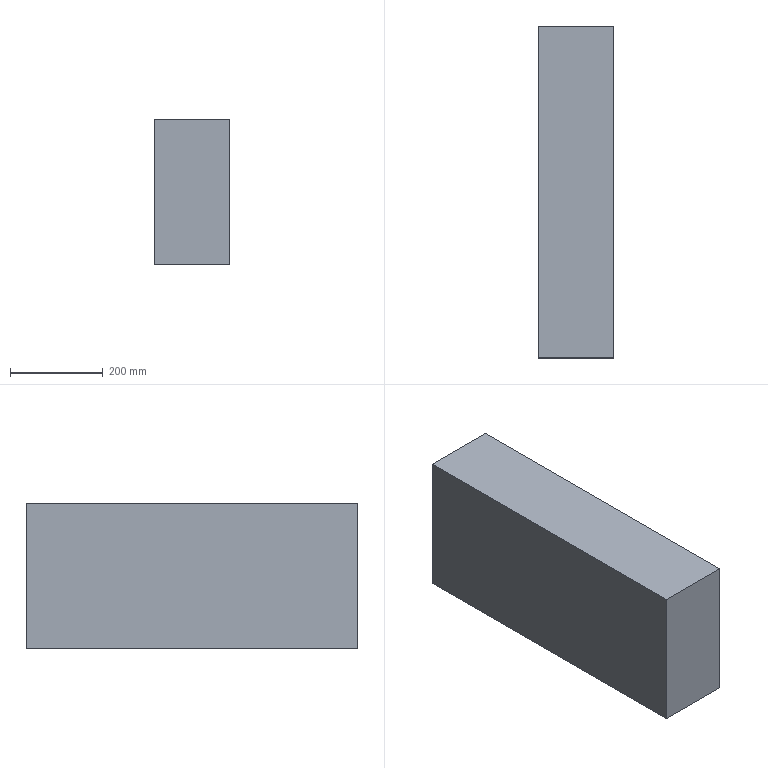Part | STEP file | 1 solid | 6 faces | box 162.496 x 714.237 x 313.918 mm | volume 36433685 mm3 | plane 6
STEP:
#1=CARTESIAN_POINT('',(0.,0.,0.));
#2=DIRECTION('',(0.,0.,1.));
#3=DIRECTION('',(1.,0.,0.));
#4=AXIS2_PLACEMENT_3D('',#1,#2,#3);
#5=CARTESIAN_POINT('',(-762.496,164.237,-106.359));
#6=VERTEX_POINT('',#5);
#7=CARTESIAN_POINT('',(-762.496,164.237,207.559));
#8=VERTEX_POINT('',#7);
#9=CARTESIAN_POINT('',(-762.496,164.237,-106.359));
#10=DIRECTION('',(0.,0.,1.));
#11=VECTOR('',#10,1.);
#12=LINE('',#9,#11);
#13=CARTESIAN_POINT('',(-762.496,164.237,207.569));
#14=DIRECTION('',(1.,0.,0.));
#15=DIRECTION('',(0.,0.,-1.));
#16=AXIS2_PLACEMENT_3D('',#13,#14,#15);
#17=PLANE('',#16);
#18=CARTESIAN_POINT('',(313.928,0.));
#19=DIRECTION('',(-1.,0.));
#20=VECTOR('',#19,1.);
#21=LINE('',#18,#20);
#22=(GEOMETRIC_REPRESENTATION_CONTEXT(2)PARAMETRIC_REPRESENTATION_CONTEXT()REPRESENTATION_CONTEXT('',''));
#23=DEFINITIONAL_REPRESENTATION('',(#21),#22);
#24=PCURVE('',#17,#23);
#25=CARTESIAN_POINT('',(-812.,164.237,-106.359));
#26=DIRECTION('',(0.,-1.,0.));
#27=DIRECTION('',(0.,0.,-1.));
#28=AXIS2_PLACEMENT_3D('',#25,#26,#27);
#29=PLANE('',#28);
#30=CARTESIAN_POINT('',(0.,49.504));
#31=DIRECTION('',(-1.,0.));
#32=VECTOR('',#31,1.);
#33=LINE('',#30,#32);
#34=(GEOMETRIC_REPRESENTATION_CONTEXT(2)PARAMETRIC_REPRESENTATION_CONTEXT()REPRESENTATION_CONTEXT('',''));
#35=DEFINITIONAL_REPRESENTATION('',(#33),#34);
#36=PCURVE('',#29,#35);
#37=SURFACE_CURVE('',#12,(#24,#36),.PCURVE_S1.);
#38=EDGE_CURVE('',#6,#8,#37,.T.);
#39=ORIENTED_EDGE('',*,*,#38,.F.);
#40=CARTESIAN_POINT('',(-762.496,-550.,-106.359));
#41=VERTEX_POINT('',#40);
#42=CARTESIAN_POINT('',(-762.496,-550.,-106.359));
#43=DIRECTION('',(0.,1.,0.));
#44=VECTOR('',#43,1.);
#45=LINE('',#42,#44);
#46=CARTESIAN_POINT('',(313.928,-714.237));
#47=DIRECTION('',(0.,1.));
#48=VECTOR('',#47,1.);
#49=LINE('',#46,#48);
#50=(GEOMETRIC_REPRESENTATION_CONTEXT(2)PARAMETRIC_REPRESENTATION_CONTEXT()REPRESENTATION_CONTEXT('',''));
#51=DEFINITIONAL_REPRESENTATION('',(#49),#50);
#52=PCURVE('',#17,#51);
#53=CARTESIAN_POINT('',(-812.,-550.,-106.359));
#54=DIRECTION('',(0.,0.,1.));
#55=DIRECTION('',(1.,0.,0.));
#56=AXIS2_PLACEMENT_3D('',#53,#54,#55);
#57=PLANE('',#56);
#58=CARTESIAN_POINT('',(49.504,0.));
#59=DIRECTION('',(0.,1.));
#60=VECTOR('',#59,1.);
#61=LINE('',#58,#60);
#62=(GEOMETRIC_REPRESENTATION_CONTEXT(2)PARAMETRIC_REPRESENTATION_CONTEXT()REPRESENTATION_CONTEXT('',''));
#63=DEFINITIONAL_REPRESENTATION('',(#61),#62);
#64=PCURVE('',#57,#63);
#65=SURFACE_CURVE('',#45,(#52,#64),.PCURVE_S1.);
#66=EDGE_CURVE('',#41,#6,#65,.T.);
#67=ORIENTED_EDGE('',*,*,#66,.F.);
#68=CARTESIAN_POINT('',(-762.496,-550.,207.559));
#69=VERTEX_POINT('',#68);
#70=CARTESIAN_POINT('',(-762.496,-550.,-106.359));
#71=DIRECTION('',(0.,0.,-1.));
#72=VECTOR('',#71,1.);
#73=LINE('',#70,#72);
#74=CARTESIAN_POINT('',(313.928,-714.237));
#75=DIRECTION('',(1.,0.));
#76=VECTOR('',#75,1.);
#77=LINE('',#74,#76);
#78=(GEOMETRIC_REPRESENTATION_CONTEXT(2)PARAMETRIC_REPRESENTATION_CONTEXT()REPRESENTATION_CONTEXT('',''));
#79=DEFINITIONAL_REPRESENTATION('',(#77),#78);
#80=PCURVE('',#17,#79);
#81=CARTESIAN_POINT('',(-812.,-550.,-106.359));
#82=DIRECTION('',(0.,1.,0.));
#83=DIRECTION('',(0.,0.,1.));
#84=AXIS2_PLACEMENT_3D('',#81,#82,#83);
#85=PLANE('',#84);
#86=CARTESIAN_POINT('',(0.,49.504));
#87=DIRECTION('',(-1.,0.));
#88=VECTOR('',#87,1.);
#89=LINE('',#86,#88);
#90=(GEOMETRIC_REPRESENTATION_CONTEXT(2)PARAMETRIC_REPRESENTATION_CONTEXT()REPRESENTATION_CONTEXT('',''));
#91=DEFINITIONAL_REPRESENTATION('',(#89),#90);
#92=PCURVE('',#85,#91);
#93=SURFACE_CURVE('',#73,(#80,#92),.PCURVE_S1.);
#94=EDGE_CURVE('',#69,#41,#93,.T.);
#95=ORIENTED_EDGE('',*,*,#94,.F.);
#96=CARTESIAN_POINT('',(-762.496,-550.,207.559));
#97=DIRECTION('',(0.,-1.,0.));
#98=VECTOR('',#97,1.);
#99=LINE('',#96,#98);
#100=CARTESIAN_POINT('',(0.01,-714.237));
#101=DIRECTION('',(0.,-1.));
#102=VECTOR('',#101,1.);
#103=LINE('',#100,#102);
#104=(GEOMETRIC_REPRESENTATION_CONTEXT(2)PARAMETRIC_REPRESENTATION_CONTEXT()REPRESENTATION_CONTEXT('',''));
#105=DEFINITIONAL_REPRESENTATION('',(#103),#104);
#106=PCURVE('',#17,#105);
#107=CARTESIAN_POINT('',(-812.,-550.,207.559));
#108=DIRECTION('',(0.,0.,-1.));
#109=DIRECTION('',(-1.,0.,0.));
#110=AXIS2_PLACEMENT_3D('',#107,#108,#109);
#111=PLANE('',#110);
#112=CARTESIAN_POINT('',(-49.504,0.));
#113=DIRECTION('',(0.,-1.));
#114=VECTOR('',#113,1.);
#115=LINE('',#112,#114);
#116=(GEOMETRIC_REPRESENTATION_CONTEXT(2)PARAMETRIC_REPRESENTATION_CONTEXT()REPRESENTATION_CONTEXT('',''));
#117=DEFINITIONAL_REPRESENTATION('',(#115),#116);
#118=PCURVE('',#111,#117);
#119=SURFACE_CURVE('',#99,(#106,#118),.PCURVE_S1.);
#120=EDGE_CURVE('',#8,#69,#119,.T.);
#121=ORIENTED_EDGE('',*,*,#120,.F.);
#122=EDGE_LOOP('',(#39,#67,#95,#121));
#123=FACE_BOUND('',#122,.T.);
#124=ADVANCED_FACE('',(#123),#17,.F.);
#125=CARTESIAN_POINT('',(-600.,164.237,-106.359));
#126=VERTEX_POINT('',#125);
#127=CARTESIAN_POINT('',(-812.,164.237,-106.359));
#128=DIRECTION('',(1.,0.,0.));
#129=VECTOR('',#128,1.);
#130=LINE('',#127,#129);
#131=CARTESIAN_POINT('',(0.,0.));
#132=DIRECTION('',(0.,1.));
#133=VECTOR('',#132,1.);
#134=LINE('',#131,#133);
#135=(GEOMETRIC_REPRESENTATION_CONTEXT(2)PARAMETRIC_REPRESENTATION_CONTEXT()REPRESENTATION_CONTEXT('',''));
#136=DEFINITIONAL_REPRESENTATION('',(#134),#135);
#137=PCURVE('',#29,#136);
#138=CARTESIAN_POINT('',(0.,714.237));
#139=DIRECTION('',(1.,0.));
#140=VECTOR('',#139,1.);
#141=LINE('',#138,#140);
#142=(GEOMETRIC_REPRESENTATION_CONTEXT(2)PARAMETRIC_REPRESENTATION_CONTEXT()REPRESENTATION_CONTEXT('',''));
#143=DEFINITIONAL_REPRESENTATION('',(#141),#142);
#144=PCURVE('',#57,#143);
#145=SURFACE_CURVE('',#130,(#137,#144),.PCURVE_S1.);
#146=EDGE_CURVE('',#6,#126,#145,.T.);
#147=ORIENTED_EDGE('',*,*,#146,.F.);
#148=ORIENTED_EDGE('',*,*,#38,.T.);
#149=CARTESIAN_POINT('',(-600.,164.237,207.559));
#150=VERTEX_POINT('',#149);
#151=CARTESIAN_POINT('',(-812.,164.237,207.559));
#152=DIRECTION('',(1.,0.,0.));
#153=VECTOR('',#152,1.);
#154=LINE('',#151,#153);
#155=CARTESIAN_POINT('',(-313.918,0.));
#156=DIRECTION('',(0.,1.));
#157=VECTOR('',#156,1.);
#158=LINE('',#155,#157);
#159=(GEOMETRIC_REPRESENTATION_CONTEXT(2)PARAMETRIC_REPRESENTATION_CONTEXT()REPRESENTATION_CONTEXT('',''));
#160=DEFINITIONAL_REPRESENTATION('',(#158),#159);
#161=PCURVE('',#29,#160);
#162=CARTESIAN_POINT('',(0.,714.237));
#163=DIRECTION('',(-1.,0.));
#164=VECTOR('',#163,1.);
#165=LINE('',#162,#164);
#166=(GEOMETRIC_REPRESENTATION_CONTEXT(2)PARAMETRIC_REPRESENTATION_CONTEXT()REPRESENTATION_CONTEXT('',''));
#167=DEFINITIONAL_REPRESENTATION('',(#165),#166);
#168=PCURVE('',#111,#167);
#169=SURFACE_CURVE('',#154,(#161,#168),.PCURVE_S1.);
#170=EDGE_CURVE('',#8,#150,#169,.T.);
#171=ORIENTED_EDGE('',*,*,#170,.T.);
#172=CARTESIAN_POINT('',(-600.,164.237,-106.359));
#173=DIRECTION('',(0.,0.,-1.));
#174=VECTOR('',#173,1.);
#175=LINE('',#172,#174);
#176=CARTESIAN_POINT('',(0.,212.));
#177=DIRECTION('',(1.,0.));
#178=VECTOR('',#177,1.);
#179=LINE('',#176,#178);
#180=(GEOMETRIC_REPRESENTATION_CONTEXT(2)PARAMETRIC_REPRESENTATION_CONTEXT()REPRESENTATION_CONTEXT('',''));
#181=DEFINITIONAL_REPRESENTATION('',(#179),#180);
#182=PCURVE('',#29,#181);
#183=CARTESIAN_POINT('',(-600.,0.,0.));
#184=DIRECTION('',(1.,0.,0.));
#185=DIRECTION('',(0.,0.,-1.));
#186=AXIS2_PLACEMENT_3D('',#183,#184,#185);
#187=PLANE('',#186);
#188=CARTESIAN_POINT('',(106.359,164.237));
#189=DIRECTION('',(1.,0.));
#190=VECTOR('',#189,1.);
#191=LINE('',#188,#190);
#192=(GEOMETRIC_REPRESENTATION_CONTEXT(2)PARAMETRIC_REPRESENTATION_CONTEXT()REPRESENTATION_CONTEXT('',''));
#193=DEFINITIONAL_REPRESENTATION('',(#191),#192);
#194=PCURVE('',#187,#193);
#195=SURFACE_CURVE('',#175,(#182,#194),.PCURVE_S1.);
#196=EDGE_CURVE('',#150,#126,#195,.T.);
#197=ORIENTED_EDGE('',*,*,#196,.T.);
#198=EDGE_LOOP('',(#147,#148,#171,#197));
#199=FACE_BOUND('',#198,.T.);
#200=ADVANCED_FACE('',(#199),#29,.F.);
#201=CARTESIAN_POINT('',(-600.,-550.,-106.359));
#202=VERTEX_POINT('',#201);
#203=CARTESIAN_POINT('',(-812.,-550.,-106.359));
#204=DIRECTION('',(1.,0.,0.));
#205=VECTOR('',#204,1.);
#206=LINE('',#203,#205);
#207=CARTESIAN_POINT('',(0.,0.));
#208=DIRECTION('',(1.,0.));
#209=VECTOR('',#208,1.);
#210=LINE('',#207,#209);
#211=(GEOMETRIC_REPRESENTATION_CONTEXT(2)PARAMETRIC_REPRESENTATION_CONTEXT()REPRESENTATION_CONTEXT('',''));
#212=DEFINITIONAL_REPRESENTATION('',(#210),#211);
#213=PCURVE('',#57,#212);
#214=CARTESIAN_POINT('',(0.,0.));
#215=DIRECTION('',(0.,1.));
#216=VECTOR('',#215,1.);
#217=LINE('',#214,#216);
#218=(GEOMETRIC_REPRESENTATION_CONTEXT(2)PARAMETRIC_REPRESENTATION_CONTEXT()REPRESENTATION_CONTEXT('',''));
#219=DEFINITIONAL_REPRESENTATION('',(#217),#218);
#220=PCURVE('',#85,#219);
#221=SURFACE_CURVE('',#206,(#213,#220),.PCURVE_S1.);
#222=EDGE_CURVE('',#41,#202,#221,.T.);
#223=ORIENTED_EDGE('',*,*,#222,.F.);
#224=ORIENTED_EDGE('',*,*,#66,.T.);
#225=ORIENTED_EDGE('',*,*,#146,.T.);
#226=CARTESIAN_POINT('',(-600.,-550.,-106.359));
#227=DIRECTION('',(0.,-1.,0.));
#228=VECTOR('',#227,1.);
#229=LINE('',#226,#228);
#230=CARTESIAN_POINT('',(212.,0.));
#231=DIRECTION('',(0.,-1.));
#232=VECTOR('',#231,1.);
#233=LINE('',#230,#232);
#234=(GEOMETRIC_REPRESENTATION_CONTEXT(2)PARAMETRIC_REPRESENTATION_CONTEXT()REPRESENTATION_CONTEXT('',''));
#235=DEFINITIONAL_REPRESENTATION('',(#233),#234);
#236=PCURVE('',#57,#235);
#237=CARTESIAN_POINT('',(106.359,-550.));
#238=DIRECTION('',(0.,-1.));
#239=VECTOR('',#238,1.);
#240=LINE('',#237,#239);
#241=(GEOMETRIC_REPRESENTATION_CONTEXT(2)PARAMETRIC_REPRESENTATION_CONTEXT()REPRESENTATION_CONTEXT('',''));
#242=DEFINITIONAL_REPRESENTATION('',(#240),#241);
#243=PCURVE('',#187,#242);
#244=SURFACE_CURVE('',#229,(#236,#243),.PCURVE_S1.);
#245=EDGE_CURVE('',#126,#202,#244,.T.);
#246=ORIENTED_EDGE('',*,*,#245,.T.);
#247=EDGE_LOOP('',(#223,#224,#225,#246));
#248=FACE_BOUND('',#247,.T.);
#249=ADVANCED_FACE('',(#248),#57,.F.);
#250=ORIENTED_EDGE('',*,*,#170,.F.);
#251=ORIENTED_EDGE('',*,*,#120,.T.);
#252=CARTESIAN_POINT('',(-600.,-550.,207.559));
#253=VERTEX_POINT('',#252);
#254=CARTESIAN_POINT('',(-812.,-550.,207.559));
#255=DIRECTION('',(1.,0.,0.));
#256=VECTOR('',#255,1.);
#257=LINE('',#254,#256);
#258=CARTESIAN_POINT('',(0.,0.));
#259=DIRECTION('',(-1.,0.));
#260=VECTOR('',#259,1.);
#261=LINE('',#258,#260);
#262=(GEOMETRIC_REPRESENTATION_CONTEXT(2)PARAMETRIC_REPRESENTATION_CONTEXT()REPRESENTATION_CONTEXT('',''));
#263=DEFINITIONAL_REPRESENTATION('',(#261),#262);
#264=PCURVE('',#111,#263);
#265=CARTESIAN_POINT('',(313.918,0.));
#266=DIRECTION('',(0.,1.));
#267=VECTOR('',#266,1.);
#268=LINE('',#265,#267);
#269=(GEOMETRIC_REPRESENTATION_CONTEXT(2)PARAMETRIC_REPRESENTATION_CONTEXT()REPRESENTATION_CONTEXT('',''));
#270=DEFINITIONAL_REPRESENTATION('',(#268),#269);
#271=PCURVE('',#85,#270);
#272=SURFACE_CURVE('',#257,(#264,#271),.PCURVE_S1.);
#273=EDGE_CURVE('',#69,#253,#272,.T.);
#274=ORIENTED_EDGE('',*,*,#273,.T.);
#275=CARTESIAN_POINT('',(-600.,-550.,207.559));
#276=DIRECTION('',(0.,1.,0.));
#277=VECTOR('',#276,1.);
#278=LINE('',#275,#277);
#279=CARTESIAN_POINT('',(-212.,0.));
#280=DIRECTION('',(0.,1.));
#281=VECTOR('',#280,1.);
#282=LINE('',#279,#281);
#283=(GEOMETRIC_REPRESENTATION_CONTEXT(2)PARAMETRIC_REPRESENTATION_CONTEXT()REPRESENTATION_CONTEXT('',''));
#284=DEFINITIONAL_REPRESENTATION('',(#282),#283);
#285=PCURVE('',#111,#284);
#286=CARTESIAN_POINT('',(-207.559,-550.));
#287=DIRECTION('',(0.,1.));
#288=VECTOR('',#287,1.);
#289=LINE('',#286,#288);
#290=(GEOMETRIC_REPRESENTATION_CONTEXT(2)PARAMETRIC_REPRESENTATION_CONTEXT()REPRESENTATION_CONTEXT('',''));
#291=DEFINITIONAL_REPRESENTATION('',(#289),#290);
#292=PCURVE('',#187,#291);
#293=SURFACE_CURVE('',#278,(#285,#292),.PCURVE_S1.);
#294=EDGE_CURVE('',#253,#150,#293,.T.);
#295=ORIENTED_EDGE('',*,*,#294,.T.);
#296=EDGE_LOOP('',(#250,#251,#274,#295));
#297=FACE_BOUND('',#296,.T.);
#298=ADVANCED_FACE('',(#297),#111,.F.);
#299=ORIENTED_EDGE('',*,*,#245,.F.);
#300=ORIENTED_EDGE('',*,*,#196,.F.);
#301=ORIENTED_EDGE('',*,*,#294,.F.);
#302=CARTESIAN_POINT('',(-600.,-550.,-106.359));
#303=DIRECTION('',(0.,0.,1.));
#304=VECTOR('',#303,1.);
#305=LINE('',#302,#304);
#306=CARTESIAN_POINT('',(106.359,-550.));
#307=DIRECTION('',(-1.,0.));
#308=VECTOR('',#307,1.);
#309=LINE('',#306,#308);
#310=(GEOMETRIC_REPRESENTATION_CONTEXT(2)PARAMETRIC_REPRESENTATION_CONTEXT()REPRESENTATION_CONTEXT('',''));
#311=DEFINITIONAL_REPRESENTATION('',(#309),#310);
#312=PCURVE('',#187,#311);
#313=CARTESIAN_POINT('',(0.,212.));
#314=DIRECTION('',(1.,0.));
#315=VECTOR('',#314,1.);
#316=LINE('',#313,#315);
#317=(GEOMETRIC_REPRESENTATION_CONTEXT(2)PARAMETRIC_REPRESENTATION_CONTEXT()REPRESENTATION_CONTEXT('',''));
#318=DEFINITIONAL_REPRESENTATION('',(#316),#317);
#319=PCURVE('',#85,#318);
#320=SURFACE_CURVE('',#305,(#312,#319),.PCURVE_S1.);
#321=EDGE_CURVE('',#202,#253,#320,.T.);
#322=ORIENTED_EDGE('',*,*,#321,.F.);
#323=EDGE_LOOP('',(#299,#300,#301,#322));
#324=FACE_BOUND('',#323,.T.);
#325=ADVANCED_FACE('',(#324),#187,.T.);
#326=ORIENTED_EDGE('',*,*,#273,.F.);
#327=ORIENTED_EDGE('',*,*,#94,.T.);
#328=ORIENTED_EDGE('',*,*,#222,.T.);
#329=ORIENTED_EDGE('',*,*,#321,.T.);
#330=EDGE_LOOP('',(#326,#327,#328,#329));
#331=FACE_BOUND('',#330,.T.);
#332=ADVANCED_FACE('',(#331),#85,.F.);
#333=CLOSED_SHELL('',(#124,#200,#249,#298,#325,#332));
#334=MANIFOLD_SOLID_BREP('',#333);
#335=(LENGTH_UNIT()NAMED_UNIT(*)SI_UNIT(.MILLI.,.METRE.));
#336=UNCERTAINTY_MEASURE_WITH_UNIT(LENGTH_MEASURE(0.0000001),#335,'','');
#337=(NAMED_UNIT(*)PLANE_ANGLE_UNIT()SI_UNIT($,.RADIAN.));
#338=(NAMED_UNIT(*)SI_UNIT($,.STERADIAN.)SOLID_ANGLE_UNIT());
#339=(GEOMETRIC_REPRESENTATION_CONTEXT(3)GLOBAL_UNCERTAINTY_ASSIGNED_CONTEXT((#336))GLOBAL_UNIT_ASSIGNED_CONTEXT((#335,#337,#338))REPRESENTATION_CONTEXT('',''));
#340=ADVANCED_BREP_SHAPE_REPRESENTATION('',(#4,#334),#339);